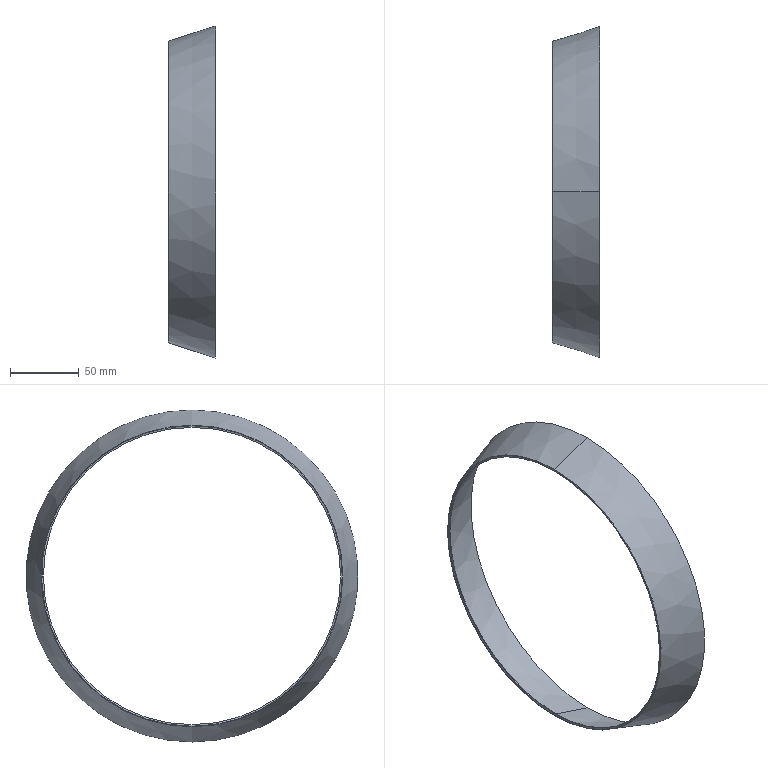Part | SolidWorks | features BaseBody 1 | 1 solid | 16 faces | box 34.434 x 242.32 x 242.32 mm | volume 26377 mm3 | cone 12 | torus 4
STEP:
#1=CARTESIAN_POINT('',(0.03978,0.,110.013));
#2=VERTEX_POINT('',#1);
#3=CARTESIAN_POINT('',(33.989,0.,121.16));
#4=VERTEX_POINT('',#3);
#5=CARTESIAN_POINT('',(0.03978,0.,110.013));
#6=DIRECTION('',(0.9501,0.,0.312));
#7=VECTOR('',#6,1000.);
#8=LINE('',#5,#7);
#9=EDGE_CURVE('',#2,#4,#8,.T.);
#10=ORIENTED_EDGE('',*,*,#9,.F.);
#11=CARTESIAN_POINT('',(0.03978,-104.628,-33.996));
#12=VERTEX_POINT('',#11);
#13=CARTESIAN_POINT('',(0.03978,0.,0.));
#14=DIRECTION('',(1.,0.,0.));
#15=DIRECTION('',(0.,0.,-1.));
#16=AXIS2_PLACEMENT_3D('',#13,#14,#15);
#17=CIRCLE('',#16,110.013);
#18=EDGE_CURVE('',#2,#12,#17,.T.);
#19=ORIENTED_EDGE('',*,*,#18,.T.);
#20=CARTESIAN_POINT('',(0.03978,0.,-110.013));
#21=VERTEX_POINT('',#20);
#22=CARTESIAN_POINT('',(0.03978,0.,0.));
#23=DIRECTION('',(1.,0.,0.));
#24=DIRECTION('',(0.,0.,-1.));
#25=AXIS2_PLACEMENT_3D('',#22,#23,#24);
#26=CIRCLE('',#25,110.013);
#27=EDGE_CURVE('',#12,#21,#26,.T.);
#28=ORIENTED_EDGE('',*,*,#27,.T.);
#29=CARTESIAN_POINT('',(33.989,0.,-121.16));
#30=VERTEX_POINT('',#29);
#31=CARTESIAN_POINT('',(0.03978,0.,-110.013));
#32=DIRECTION('',(0.9501,0.,-0.312));
#33=VECTOR('',#32,1000.);
#34=LINE('',#31,#33);
#35=EDGE_CURVE('',#21,#30,#34,.T.);
#36=ORIENTED_EDGE('',*,*,#35,.T.);
#37=CARTESIAN_POINT('',(33.989,0.,0.));
#38=DIRECTION('',(1.,0.,0.));
#39=DIRECTION('',(0.,0.,-1.));
#40=AXIS2_PLACEMENT_3D('',#37,#38,#39);
#41=CIRCLE('',#40,121.16);
#42=EDGE_CURVE('',#4,#30,#41,.T.);
#43=ORIENTED_EDGE('',*,*,#42,.F.);
#44=EDGE_LOOP('',(#10,#19,#28,#36,#43));
#45=FACE_OUTER_BOUND('',#44,.T.);
#46=CARTESIAN_POINT('',(33.989,0.,0.));
#47=DIRECTION('',(1.,0.,0.));
#48=DIRECTION('',(0.,1.,0.));
#49=AXIS2_PLACEMENT_3D('',#46,#47,#48);
#50=CONICAL_SURFACE('',#49,121.16,0.3173);
#51=ADVANCED_FACE('',(#45),#50,.T.);
#52=CARTESIAN_POINT('',(34.268,0.,-120.199));
#53=VERTEX_POINT('',#52);
#54=CARTESIAN_POINT('',(34.268,0.,-120.199));
#55=DIRECTION('',(-0.2785,0.,-0.9604));
#56=VECTOR('',#55,1000.);
#57=LINE('',#54,#56);
#58=EDGE_CURVE('',#53,#30,#57,.T.);
#59=ORIENTED_EDGE('',*,*,#58,.F.);
#60=CARTESIAN_POINT('',(34.268,0.,120.199));
#61=VERTEX_POINT('',#60);
#62=CARTESIAN_POINT('',(34.268,0.,0.));
#63=DIRECTION('',(1.,0.,0.));
#64=DIRECTION('',(0.,0.,-1.));
#65=AXIS2_PLACEMENT_3D('',#62,#63,#64);
#66=CIRCLE('',#65,120.199);
#67=EDGE_CURVE('',#61,#53,#66,.T.);
#68=ORIENTED_EDGE('',*,*,#67,.F.);
#69=CARTESIAN_POINT('',(34.268,0.,120.199));
#70=DIRECTION('',(-0.2785,0.,0.9604));
#71=VECTOR('',#70,1000.);
#72=LINE('',#69,#71);
#73=EDGE_CURVE('',#61,#4,#72,.T.);
#74=ORIENTED_EDGE('',*,*,#73,.T.);
#75=ORIENTED_EDGE('',*,*,#42,.T.);
#76=EDGE_LOOP('',(#59,#68,#74,#75));
#77=FACE_OUTER_BOUND('',#76,.T.);
#78=CARTESIAN_POINT('',(34.268,0.,0.));
#79=DIRECTION('',(-1.,0.,0.));
#80=DIRECTION('',(0.,1.,0.));
#81=AXIS2_PLACEMENT_3D('',#78,#79,#80);
#82=CONICAL_SURFACE('',#81,120.199,1.289);
#83=ADVANCED_FACE('',(#77),#82,.T.);
#84=ORIENTED_EDGE('',*,*,#58,.T.);
#85=CARTESIAN_POINT('',(33.989,0.,0.));
#86=DIRECTION('',(1.,0.,0.));
#87=DIRECTION('',(0.,0.,-1.));
#88=AXIS2_PLACEMENT_3D('',#85,#86,#87);
#89=CIRCLE('',#88,121.16);
#90=EDGE_CURVE('',#30,#4,#89,.T.);
#91=ORIENTED_EDGE('',*,*,#90,.T.);
#92=ORIENTED_EDGE('',*,*,#73,.F.);
#93=CARTESIAN_POINT('',(34.268,0.,0.));
#94=DIRECTION('',(1.,0.,0.));
#95=DIRECTION('',(0.,0.,-1.));
#96=AXIS2_PLACEMENT_3D('',#93,#94,#95);
#97=CIRCLE('',#96,120.199);
#98=EDGE_CURVE('',#53,#61,#97,.T.);
#99=ORIENTED_EDGE('',*,*,#98,.F.);
#100=EDGE_LOOP('',(#84,#91,#92,#99));
#101=FACE_OUTER_BOUND('',#100,.T.);
#102=CARTESIAN_POINT('',(34.268,0.,0.));
#103=DIRECTION('',(-1.,0.,0.));
#104=DIRECTION('',(0.,-1.,0.));
#105=AXIS2_PLACEMENT_3D('',#102,#103,#104);
#106=CONICAL_SURFACE('',#105,120.199,1.289);
#107=ADVANCED_FACE('',(#101),#106,.T.);
#108=CARTESIAN_POINT('',(1.177,0.,109.334));
#109=VERTEX_POINT('',#108);
#110=CARTESIAN_POINT('',(1.177,0.,109.334));
#111=DIRECTION('',(0.9501,0.,0.312));
#112=VECTOR('',#111,1000.);
#113=LINE('',#110,#112);
#114=EDGE_CURVE('',#109,#61,#113,.T.);
#115=ORIENTED_EDGE('',*,*,#114,.F.);
#116=CARTESIAN_POINT('',(1.177,103.983,33.786));
#117=VERTEX_POINT('',#116);
#118=CARTESIAN_POINT('',(1.177,0.,0.));
#119=DIRECTION('',(1.,0.,0.));
#120=DIRECTION('',(0.,0.,-1.));
#121=AXIS2_PLACEMENT_3D('',#118,#119,#120);
#122=CIRCLE('',#121,109.334);
#123=EDGE_CURVE('',#117,#109,#122,.T.);
#124=ORIENTED_EDGE('',*,*,#123,.F.);
#125=CARTESIAN_POINT('',(1.177,0.,-109.334));
#126=VERTEX_POINT('',#125);
#127=CARTESIAN_POINT('',(1.177,0.,0.));
#128=DIRECTION('',(1.,0.,0.));
#129=DIRECTION('',(0.,0.,-1.));
#130=AXIS2_PLACEMENT_3D('',#127,#128,#129);
#131=CIRCLE('',#130,109.334);
#132=EDGE_CURVE('',#126,#117,#131,.T.);
#133=ORIENTED_EDGE('',*,*,#132,.F.);
#134=CARTESIAN_POINT('',(1.177,0.,-109.334));
#135=DIRECTION('',(0.9501,0.,-0.312));
#136=VECTOR('',#135,1000.);
#137=LINE('',#134,#136);
#138=EDGE_CURVE('',#126,#53,#137,.T.);
#139=ORIENTED_EDGE('',*,*,#138,.T.);
#140=ORIENTED_EDGE('',*,*,#98,.T.);
#141=EDGE_LOOP('',(#115,#124,#133,#139,#140));
#142=FACE_OUTER_BOUND('',#141,.T.);
#143=CARTESIAN_POINT('',(1.177,0.,0.));
#144=DIRECTION('',(1.,0.,0.));
#145=DIRECTION('',(0.,-1.,0.));
#146=AXIS2_PLACEMENT_3D('',#143,#144,#145);
#147=CONICAL_SURFACE('',#146,109.334,0.3173);
#148=ADVANCED_FACE('',(#142),#147,.F.);
#149=ORIENTED_EDGE('',*,*,#114,.T.);
#150=ORIENTED_EDGE('',*,*,#67,.T.);
#151=ORIENTED_EDGE('',*,*,#138,.F.);
#152=CARTESIAN_POINT('',(1.177,-103.983,-33.786));
#153=VERTEX_POINT('',#152);
#154=CARTESIAN_POINT('',(1.177,0.,0.));
#155=DIRECTION('',(1.,0.,0.));
#156=DIRECTION('',(0.,0.,-1.));
#157=AXIS2_PLACEMENT_3D('',#154,#155,#156);
#158=CIRCLE('',#157,109.334);
#159=EDGE_CURVE('',#153,#126,#158,.T.);
#160=ORIENTED_EDGE('',*,*,#159,.F.);
#161=CARTESIAN_POINT('',(1.177,0.,0.));
#162=DIRECTION('',(1.,0.,0.));
#163=DIRECTION('',(0.,0.,-1.));
#164=AXIS2_PLACEMENT_3D('',#161,#162,#163);
#165=CIRCLE('',#164,109.334);
#166=EDGE_CURVE('',#109,#153,#165,.T.);
#167=ORIENTED_EDGE('',*,*,#166,.F.);
#168=EDGE_LOOP('',(#149,#150,#151,#160,#167));
#169=FACE_OUTER_BOUND('',#168,.T.);
#170=CARTESIAN_POINT('',(1.177,0.,0.));
#171=DIRECTION('',(1.,0.,0.));
#172=DIRECTION('',(0.,1.,0.));
#173=AXIS2_PLACEMENT_3D('',#170,#171,#172);
#174=CONICAL_SURFACE('',#173,109.334,0.3173);
#175=ADVANCED_FACE('',(#169),#174,.F.);
#176=CARTESIAN_POINT('',(1.048,-103.749,-33.71));
#177=VERTEX_POINT('',#176);
#178=CARTESIAN_POINT('',(1.24,-103.802,-33.727));
#179=DIRECTION('',(0.,0.309,-0.9511));
#180=DIRECTION('',(-0.312,-0.9036,-0.2936));
#181=AXIS2_PLACEMENT_3D('',#178,#179,#180);
#182=CIRCLE('',#181,0.2);
#183=EDGE_CURVE('',#153,#177,#182,.T.);
#184=ORIENTED_EDGE('',*,*,#183,.T.);
#185=CARTESIAN_POINT('',(1.048,0.,109.088));
#186=VERTEX_POINT('',#185);
#187=CARTESIAN_POINT('',(1.048,0.,109.088));
#188=CARTESIAN_POINT('',(1.048,-8.568,109.088));
#189=CARTESIAN_POINT('',(1.048,-17.135,108.074));
#190=CARTESIAN_POINT('',(1.048,-33.797,104.074));
#191=CARTESIAN_POINT('',(1.048,-41.891,101.088));
#192=CARTESIAN_POINT('',(1.048,-57.159,93.308));
#193=CARTESIAN_POINT('',(1.048,-64.332,88.515));
#194=CARTESIAN_POINT('',(1.048,-77.362,77.387));
#195=CARTESIAN_POINT('',(1.048,-83.218,71.052));
#196=CARTESIAN_POINT('',(1.048,-93.29,57.189));
#197=CARTESIAN_POINT('',(1.048,-97.505,49.662));
#198=CARTESIAN_POINT('',(1.048,-104.063,33.831));
#199=CARTESIAN_POINT('',(1.048,-106.405,25.527));
#200=CARTESIAN_POINT('',(1.048,-109.085,8.603));
#201=CARTESIAN_POINT('',(1.048,-109.424,-0.01761));
#202=CARTESIAN_POINT('',(1.048,-108.079,-17.1));
#203=CARTESIAN_POINT('',(1.048,-106.396,-25.562));
#204=CARTESIAN_POINT('',(1.048,-103.749,-33.71));
#205=B_SPLINE_CURVE_WITH_KNOTS('',3,(#187,#188,#189,#190,#191,#192,#193,#194,#195,#196,#197,#198,#199,#200,#201,#202,#203,#204),.UNSPECIFIED.,.F.,.F.,(4,2,2,2,2,2,2,2,4),(0.,0.2356,0.4712,0.7069,0.9425,1.178,1.414,1.649,1.885),.UNSPECIFIED.);
#206=EDGE_CURVE('',#186,#177,#205,.T.);
#207=ORIENTED_EDGE('',*,*,#206,.F.);
#208=CARTESIAN_POINT('',(1.048,103.749,33.71));
#209=VERTEX_POINT('',#208);
#210=CARTESIAN_POINT('',(1.048,103.749,33.71));
#211=CARTESIAN_POINT('',(1.048,101.984,39.142));
#212=CARTESIAN_POINT('',(1.048,99.791,44.436));
#213=CARTESIAN_POINT('',(1.048,94.605,54.614));
#214=CARTESIAN_POINT('',(1.048,91.611,59.499));
#215=CARTESIAN_POINT('',(1.048,84.897,68.741));
#216=CARTESIAN_POINT('',(1.048,81.176,73.098));
#217=CARTESIAN_POINT('',(1.048,73.098,81.176));
#218=CARTESIAN_POINT('',(1.048,68.741,84.897));
#219=CARTESIAN_POINT('',(1.048,59.499,91.611));
#220=CARTESIAN_POINT('',(1.048,54.614,94.605));
#221=CARTESIAN_POINT('',(1.048,44.436,99.791));
#222=CARTESIAN_POINT('',(1.048,39.142,101.984));
#223=CARTESIAN_POINT('',(1.048,28.278,105.514));
#224=CARTESIAN_POINT('',(1.048,22.707,106.851));
#225=CARTESIAN_POINT('',(1.048,11.424,108.638));
#226=CARTESIAN_POINT('',(1.048,5.712,109.088));
#227=CARTESIAN_POINT('',(1.048,0.,109.088));
#228=B_SPLINE_CURVE_WITH_KNOTS('',3,(#210,#211,#212,#213,#214,#215,#216,#217,#218,#219,#220,#221,#222,#223,#224,#225,#226,#227),.UNSPECIFIED.,.F.,.F.,(4,2,2,2,2,2,2,2,4),(0.,0.1571,0.3142,0.4712,0.6283,0.7854,0.9425,1.1,1.257),.UNSPECIFIED.);
#229=EDGE_CURVE('',#209,#186,#228,.T.);
#230=ORIENTED_EDGE('',*,*,#229,.F.);
#231=CARTESIAN_POINT('',(1.24,103.802,33.727));
#232=DIRECTION('',(0.,-0.309,0.9511));
#233=DIRECTION('',(-0.312,0.9036,0.2936));
#234=AXIS2_PLACEMENT_3D('',#231,#232,#233);
#235=CIRCLE('',#234,0.2);
#236=EDGE_CURVE('',#117,#209,#235,.T.);
#237=ORIENTED_EDGE('',*,*,#236,.F.);
#238=ORIENTED_EDGE('',*,*,#123,.T.);
#239=ORIENTED_EDGE('',*,*,#166,.T.);
#240=EDGE_LOOP('',(#184,#207,#230,#237,#238,#239));
#241=FACE_OUTER_BOUND('',#240,.T.);
#242=CARTESIAN_POINT('',(1.24,0.,0.));
#243=DIRECTION('',(1.,0.,0.));
#244=DIRECTION('',(0.,0.309,-0.9511));
#245=AXIS2_PLACEMENT_3D('',#242,#243,#244);
#246=TOROIDAL_SURFACE('',#245,109.144,0.2);
#247=ADVANCED_FACE('',(#241),#246,.F.);
#248=ORIENTED_EDGE('',*,*,#183,.F.);
#249=ORIENTED_EDGE('',*,*,#159,.T.);
#250=ORIENTED_EDGE('',*,*,#132,.T.);
#251=ORIENTED_EDGE('',*,*,#236,.T.);
#252=CARTESIAN_POINT('',(1.048,0.,-109.088));
#253=VERTEX_POINT('',#252);
#254=CARTESIAN_POINT('',(1.048,0.,0.));
#255=DIRECTION('',(1.,0.,0.));
#256=DIRECTION('',(0.,0.,-1.));
#257=AXIS2_PLACEMENT_3D('',#254,#255,#256);
#258=CIRCLE('',#257,109.088);
#259=EDGE_CURVE('',#253,#209,#258,.T.);
#260=ORIENTED_EDGE('',*,*,#259,.F.);
#261=CARTESIAN_POINT('',(1.048,-103.749,-33.71));
#262=CARTESIAN_POINT('',(1.048,-101.984,-39.142));
#263=CARTESIAN_POINT('',(1.048,-99.791,-44.436));
#264=CARTESIAN_POINT('',(1.048,-94.605,-54.614));
#265=CARTESIAN_POINT('',(1.048,-91.611,-59.499));
#266=CARTESIAN_POINT('',(1.048,-84.897,-68.741));
#267=CARTESIAN_POINT('',(1.048,-81.176,-73.098));
#268=CARTESIAN_POINT('',(1.048,-73.098,-81.176));
#269=CARTESIAN_POINT('',(1.048,-68.741,-84.897));
#270=CARTESIAN_POINT('',(1.048,-59.499,-91.611));
#271=CARTESIAN_POINT('',(1.048,-54.614,-94.605));
#272=CARTESIAN_POINT('',(1.048,-44.436,-99.791));
#273=CARTESIAN_POINT('',(1.048,-39.142,-101.984));
#274=CARTESIAN_POINT('',(1.048,-28.278,-105.514));
#275=CARTESIAN_POINT('',(1.048,-22.707,-106.851));
#276=CARTESIAN_POINT('',(1.048,-11.424,-108.638));
#277=CARTESIAN_POINT('',(1.048,-5.712,-109.088));
#278=CARTESIAN_POINT('',(1.048,0.,-109.088));
#279=B_SPLINE_CURVE_WITH_KNOTS('',3,(#261,#262,#263,#264,#265,#266,#267,#268,#269,#270,#271,#272,#273,#274,#275,#276,#277,#278),.UNSPECIFIED.,.F.,.F.,(4,2,2,2,2,2,2,2,4),(0.,0.1571,0.3142,0.4712,0.6283,0.7854,0.9425,1.1,1.257),.UNSPECIFIED.);
#280=EDGE_CURVE('',#177,#253,#279,.T.);
#281=ORIENTED_EDGE('',*,*,#280,.F.);
#282=EDGE_LOOP('',(#248,#249,#250,#251,#260,#281));
#283=FACE_OUTER_BOUND('',#282,.T.);
#284=CARTESIAN_POINT('',(1.24,0.,0.));
#285=DIRECTION('',(1.,0.,0.));
#286=DIRECTION('',(0.,-0.309,0.9511));
#287=AXIS2_PLACEMENT_3D('',#284,#285,#286);
#288=TOROIDAL_SURFACE('',#287,109.144,0.2);
#289=ADVANCED_FACE('',(#283),#288,.F.);
#290=CARTESIAN_POINT('',(1.133,0.,-108.793));
#291=VERTEX_POINT('',#290);
#292=CARTESIAN_POINT('',(1.133,0.,-108.793));
#293=DIRECTION('',(-0.2785,0.,-0.9604));
#294=VECTOR('',#293,1000.);
#295=LINE('',#292,#294);
#296=EDGE_CURVE('',#291,#253,#295,.T.);
#297=ORIENTED_EDGE('',*,*,#296,.F.);
#298=CARTESIAN_POINT('',(1.133,0.,108.793));
#299=VERTEX_POINT('',#298);
#300=CARTESIAN_POINT('',(1.133,0.,0.));
#301=DIRECTION('',(1.,0.,0.));
#302=DIRECTION('',(0.,0.,-1.));
#303=AXIS2_PLACEMENT_3D('',#300,#301,#302);
#304=CIRCLE('',#303,108.793);
#305=EDGE_CURVE('',#299,#291,#304,.T.);
#306=ORIENTED_EDGE('',*,*,#305,.F.);
#307=CARTESIAN_POINT('',(1.133,0.,108.793));
#308=DIRECTION('',(-0.2785,0.,0.9604));
#309=VECTOR('',#308,1000.);
#310=LINE('',#307,#309);
#311=EDGE_CURVE('',#299,#186,#310,.T.);
#312=ORIENTED_EDGE('',*,*,#311,.T.);
#313=ORIENTED_EDGE('',*,*,#206,.T.);
#314=ORIENTED_EDGE('',*,*,#280,.T.);
#315=EDGE_LOOP('',(#297,#306,#312,#313,#314));
#316=FACE_OUTER_BOUND('',#315,.T.);
#317=CARTESIAN_POINT('',(1.133,0.,0.));
#318=DIRECTION('',(-1.,0.,0.));
#319=DIRECTION('',(0.,1.,0.));
#320=AXIS2_PLACEMENT_3D('',#317,#318,#319);
#321=CONICAL_SURFACE('',#320,108.793,1.289);
#322=ADVANCED_FACE('',(#316),#321,.T.);
#323=ORIENTED_EDGE('',*,*,#296,.T.);
#324=ORIENTED_EDGE('',*,*,#259,.T.);
#325=ORIENTED_EDGE('',*,*,#229,.T.);
#326=ORIENTED_EDGE('',*,*,#311,.F.);
#327=CARTESIAN_POINT('',(1.133,0.,0.));
#328=DIRECTION('',(1.,0.,0.));
#329=DIRECTION('',(0.,0.,-1.));
#330=AXIS2_PLACEMENT_3D('',#327,#328,#329);
#331=CIRCLE('',#330,108.793);
#332=EDGE_CURVE('',#291,#299,#331,.T.);
#333=ORIENTED_EDGE('',*,*,#332,.F.);
#334=EDGE_LOOP('',(#323,#324,#325,#326,#333));
#335=FACE_OUTER_BOUND('',#334,.T.);
#336=CARTESIAN_POINT('',(1.133,0.,0.));
#337=DIRECTION('',(-1.,0.,0.));
#338=DIRECTION('',(0.,-1.,0.));
#339=AXIS2_PLACEMENT_3D('',#336,#337,#338);
#340=CONICAL_SURFACE('',#339,108.793,1.289);
#341=ADVANCED_FACE('',(#335),#340,.T.);
#342=CARTESIAN_POINT('',(0.1826,0.,108.481));
#343=VERTEX_POINT('',#342);
#344=CARTESIAN_POINT('',(0.1826,0.,108.481));
#345=DIRECTION('',(0.9501,0.,0.312));
#346=VECTOR('',#345,1000.);
#347=LINE('',#344,#346);
#348=EDGE_CURVE('',#343,#299,#347,.T.);
#349=ORIENTED_EDGE('',*,*,#348,.F.);
#350=CARTESIAN_POINT('',(0.1826,0.,-108.481));
#351=VERTEX_POINT('',#350);
#352=CARTESIAN_POINT('',(0.1826,0.,0.));
#353=DIRECTION('',(1.,0.,0.));
#354=DIRECTION('',(0.,0.,-1.));
#355=AXIS2_PLACEMENT_3D('',#352,#353,#354);
#356=CIRCLE('',#355,108.481);
#357=EDGE_CURVE('',#351,#343,#356,.T.);
#358=ORIENTED_EDGE('',*,*,#357,.F.);
#359=CARTESIAN_POINT('',(0.1826,0.,-108.481));
#360=DIRECTION('',(0.9501,0.,-0.312));
#361=VECTOR('',#360,1000.);
#362=LINE('',#359,#361);
#363=EDGE_CURVE('',#351,#291,#362,.T.);
#364=ORIENTED_EDGE('',*,*,#363,.T.);
#365=ORIENTED_EDGE('',*,*,#332,.T.);
#366=EDGE_LOOP('',(#349,#358,#364,#365));
#367=FACE_OUTER_BOUND('',#366,.T.);
#368=CARTESIAN_POINT('',(0.1826,0.,0.));
#369=DIRECTION('',(1.,0.,0.));
#370=DIRECTION('',(0.,-1.,0.));
#371=AXIS2_PLACEMENT_3D('',#368,#369,#370);
#372=CONICAL_SURFACE('',#371,108.481,0.3173);
#373=ADVANCED_FACE('',(#367),#372,.F.);
#374=ORIENTED_EDGE('',*,*,#348,.T.);
#375=ORIENTED_EDGE('',*,*,#305,.T.);
#376=ORIENTED_EDGE('',*,*,#363,.F.);
#377=CARTESIAN_POINT('',(0.1826,0.,0.));
#378=DIRECTION('',(1.,0.,0.));
#379=DIRECTION('',(0.,0.,-1.));
#380=AXIS2_PLACEMENT_3D('',#377,#378,#379);
#381=CIRCLE('',#380,108.481);
#382=EDGE_CURVE('',#343,#351,#381,.T.);
#383=ORIENTED_EDGE('',*,*,#382,.F.);
#384=EDGE_LOOP('',(#374,#375,#376,#383));
#385=FACE_OUTER_BOUND('',#384,.T.);
#386=CARTESIAN_POINT('',(0.1826,0.,0.));
#387=DIRECTION('',(1.,0.,0.));
#388=DIRECTION('',(0.,1.,0.));
#389=AXIS2_PLACEMENT_3D('',#386,#387,#388);
#390=CONICAL_SURFACE('',#389,108.481,0.3173);
#391=ADVANCED_FACE('',(#385),#390,.F.);
#392=CARTESIAN_POINT('',(-0.1548,0.,-109.644));
#393=VERTEX_POINT('',#392);
#394=CARTESIAN_POINT('',(0.1826,0.,-108.481));
#395=DIRECTION('',(-0.2785,0.,-0.9604));
#396=VECTOR('',#395,1000.);
#397=LINE('',#394,#396);
#398=EDGE_CURVE('',#351,#393,#397,.T.);
#399=ORIENTED_EDGE('',*,*,#398,.T.);
#400=CARTESIAN_POINT('',(-0.1548,-104.278,-33.882));
#401=VERTEX_POINT('',#400);
#402=CARTESIAN_POINT('',(-0.1548,-104.278,-33.882));
#403=CARTESIAN_POINT('',(-0.1548,-102.504,-39.342));
#404=CARTESIAN_POINT('',(-0.1548,-100.3,-44.662));
#405=CARTESIAN_POINT('',(-0.1548,-95.087,-54.893));
#406=CARTESIAN_POINT('',(-0.1548,-92.078,-59.803));
#407=CARTESIAN_POINT('',(-0.1548,-85.329,-69.092));
#408=CARTESIAN_POINT('',(-0.1548,-81.59,-73.471));
#409=CARTESIAN_POINT('',(-0.1548,-73.471,-81.59));
#410=CARTESIAN_POINT('',(-0.1548,-69.092,-85.329));
#411=CARTESIAN_POINT('',(-0.1548,-59.803,-92.078));
#412=CARTESIAN_POINT('',(-0.1548,-54.893,-95.087));
#413=CARTESIAN_POINT('',(-0.1548,-44.662,-100.3));
#414=CARTESIAN_POINT('',(-0.1548,-39.342,-102.504));
#415=CARTESIAN_POINT('',(-0.1548,-28.422,-106.052));
#416=CARTESIAN_POINT('',(-0.1548,-22.822,-107.396));
#417=CARTESIAN_POINT('',(-0.1548,-11.482,-109.192));
#418=CARTESIAN_POINT('',(-0.1548,-5.741,-109.644));
#419=CARTESIAN_POINT('',(-0.1548,0.,-109.644));
#420=B_SPLINE_CURVE_WITH_KNOTS('',3,(#402,#403,#404,#405,#406,#407,#408,#409,#410,#411,#412,#413,#414,#415,#416,#417,#418,#419),.UNSPECIFIED.,.F.,.F.,(4,2,2,2,2,2,2,2,4),(0.,0.1571,0.3142,0.4712,0.6283,0.7854,0.9425,1.1,1.257),.UNSPECIFIED.);
#421=EDGE_CURVE('',#401,#393,#420,.T.);
#422=ORIENTED_EDGE('',*,*,#421,.F.);
#423=CARTESIAN_POINT('',(-0.1548,0.,109.644));
#424=VERTEX_POINT('',#423);
#425=CARTESIAN_POINT('',(-0.1548,0.,0.));
#426=DIRECTION('',(1.,0.,0.));
#427=DIRECTION('',(0.,0.,-1.));
#428=AXIS2_PLACEMENT_3D('',#425,#426,#427);
#429=CIRCLE('',#428,109.644);
#430=EDGE_CURVE('',#424,#401,#429,.T.);
#431=ORIENTED_EDGE('',*,*,#430,.F.);
#432=CARTESIAN_POINT('',(0.1826,0.,108.481));
#433=DIRECTION('',(-0.2785,0.,0.9604));
#434=VECTOR('',#433,1000.);
#435=LINE('',#432,#434);
#436=EDGE_CURVE('',#343,#424,#435,.T.);
#437=ORIENTED_EDGE('',*,*,#436,.F.);
#438=ORIENTED_EDGE('',*,*,#382,.T.);
#439=EDGE_LOOP('',(#399,#422,#431,#437,#438));
#440=FACE_OUTER_BOUND('',#439,.T.);
#441=CARTESIAN_POINT('',(-0.1548,0.,0.));
#442=DIRECTION('',(-1.,0.,0.));
#443=DIRECTION('',(0.,1.,0.));
#444=AXIS2_PLACEMENT_3D('',#441,#442,#443);
#445=CONICAL_SURFACE('',#444,109.644,1.289);
#446=ADVANCED_FACE('',(#440),#445,.F.);
#447=ORIENTED_EDGE('',*,*,#398,.F.);
#448=ORIENTED_EDGE('',*,*,#357,.T.);
#449=ORIENTED_EDGE('',*,*,#436,.T.);
#450=CARTESIAN_POINT('',(-0.1548,104.278,33.882));
#451=VERTEX_POINT('',#450);
#452=CARTESIAN_POINT('',(-0.1548,104.278,33.882));
#453=CARTESIAN_POINT('',(-0.1548,102.504,39.342));
#454=CARTESIAN_POINT('',(-0.1548,100.3,44.662));
#455=CARTESIAN_POINT('',(-0.1548,95.087,54.893));
#456=CARTESIAN_POINT('',(-0.1548,92.078,59.803));
#457=CARTESIAN_POINT('',(-0.1548,85.329,69.092));
#458=CARTESIAN_POINT('',(-0.1548,81.59,73.471));
#459=CARTESIAN_POINT('',(-0.1548,73.471,81.59));
#460=CARTESIAN_POINT('',(-0.1548,69.092,85.329));
#461=CARTESIAN_POINT('',(-0.1548,59.803,92.078));
#462=CARTESIAN_POINT('',(-0.1548,54.893,95.087));
#463=CARTESIAN_POINT('',(-0.1548,44.662,100.3));
#464=CARTESIAN_POINT('',(-0.1548,39.342,102.504));
#465=CARTESIAN_POINT('',(-0.1548,28.422,106.052));
#466=CARTESIAN_POINT('',(-0.1548,22.822,107.396));
#467=CARTESIAN_POINT('',(-0.1548,11.482,109.192));
#468=CARTESIAN_POINT('',(-0.1548,5.741,109.644));
#469=CARTESIAN_POINT('',(-0.1548,0.,109.644));
#470=B_SPLINE_CURVE_WITH_KNOTS('',3,(#452,#453,#454,#455,#456,#457,#458,#459,#460,#461,#462,#463,#464,#465,#466,#467,#468,#469),.UNSPECIFIED.,.F.,.F.,(4,2,2,2,2,2,2,2,4),(0.,0.1571,0.3142,0.4712,0.6283,0.7854,0.9425,1.1,1.257),.UNSPECIFIED.);
#471=EDGE_CURVE('',#451,#424,#470,.T.);
#472=ORIENTED_EDGE('',*,*,#471,.F.);
#473=CARTESIAN_POINT('',(-0.1548,0.,-109.644));
#474=CARTESIAN_POINT('',(-0.1548,8.611,-109.644));
#475=CARTESIAN_POINT('',(-0.1548,17.222,-108.625));
#476=CARTESIAN_POINT('',(-0.1548,33.969,-104.604));
#477=CARTESIAN_POINT('',(-0.1548,42.105,-101.603));
#478=CARTESIAN_POINT('',(-0.1548,57.45,-93.784));
#479=CARTESIAN_POINT('',(-0.1548,64.66,-88.967));
#480=CARTESIAN_POINT('',(-0.1548,77.756,-77.781));
#481=CARTESIAN_POINT('',(-0.1548,83.642,-71.414));
#482=CARTESIAN_POINT('',(-0.1548,93.766,-57.48));
#483=CARTESIAN_POINT('',(-0.1548,98.002,-49.915));
#484=CARTESIAN_POINT('',(-0.1548,104.593,-34.003));
#485=CARTESIAN_POINT('',(-0.1548,106.947,-25.658));
#486=CARTESIAN_POINT('',(-0.1548,109.641,-8.647));
#487=CARTESIAN_POINT('',(-0.1548,109.982,0.0177));
#488=CARTESIAN_POINT('',(-0.1548,108.63,17.187));
#489=CARTESIAN_POINT('',(-0.1548,106.939,25.692));
#490=CARTESIAN_POINT('',(-0.1548,104.278,33.882));
#491=B_SPLINE_CURVE_WITH_KNOTS('',3,(#473,#474,#475,#476,#477,#478,#479,#480,#481,#482,#483,#484,#485,#486,#487,#488,#489,#490),.UNSPECIFIED.,.F.,.F.,(4,2,2,2,2,2,2,2,4),(0.,0.2356,0.4712,0.7069,0.9425,1.178,1.414,1.649,1.885),.UNSPECIFIED.);
#492=EDGE_CURVE('',#393,#451,#491,.T.);
#493=ORIENTED_EDGE('',*,*,#492,.F.);
#494=EDGE_LOOP('',(#447,#448,#449,#472,#493));
#495=FACE_OUTER_BOUND('',#494,.T.);
#496=CARTESIAN_POINT('',(-0.1548,0.,0.));
#497=DIRECTION('',(-1.,0.,0.));
#498=DIRECTION('',(0.,-1.,0.));
#499=AXIS2_PLACEMENT_3D('',#496,#497,#498);
#500=CONICAL_SURFACE('',#499,109.644,1.289);
#501=ADVANCED_FACE('',(#495),#500,.F.);
#502=CARTESIAN_POINT('',(0.1334,-104.357,-33.908));
#503=DIRECTION('',(0.,0.309,-0.9511));
#504=DIRECTION('',(-0.312,-0.9036,-0.2936));
#505=AXIS2_PLACEMENT_3D('',#502,#503,#504);
#506=CIRCLE('',#505,0.3);
#507=EDGE_CURVE('',#12,#401,#506,.T.);
#508=ORIENTED_EDGE('',*,*,#507,.T.);
#509=ORIENTED_EDGE('',*,*,#421,.T.);
#510=ORIENTED_EDGE('',*,*,#492,.T.);
#511=CARTESIAN_POINT('',(0.03978,104.628,33.996));
#512=VERTEX_POINT('',#511);
#513=CARTESIAN_POINT('',(0.1334,104.357,33.908));
#514=DIRECTION('',(0.,-0.309,0.9511));
#515=DIRECTION('',(-0.312,0.9036,0.2936));
#516=AXIS2_PLACEMENT_3D('',#513,#514,#515);
#517=CIRCLE('',#516,0.3);
#518=EDGE_CURVE('',#512,#451,#517,.T.);
#519=ORIENTED_EDGE('',*,*,#518,.F.);
#520=CARTESIAN_POINT('',(0.03978,0.,0.));
#521=DIRECTION('',(1.,0.,0.));
#522=DIRECTION('',(0.,0.,-1.));
#523=AXIS2_PLACEMENT_3D('',#520,#521,#522);
#524=CIRCLE('',#523,110.013);
#525=EDGE_CURVE('',#21,#512,#524,.T.);
#526=ORIENTED_EDGE('',*,*,#525,.F.);
#527=ORIENTED_EDGE('',*,*,#27,.F.);
#528=EDGE_LOOP('',(#508,#509,#510,#519,#526,#527));
#529=FACE_OUTER_BOUND('',#528,.T.);
#530=CARTESIAN_POINT('',(0.1334,0.,0.));
#531=DIRECTION('',(1.,0.,0.));
#532=DIRECTION('',(0.,-0.309,0.9511));
#533=AXIS2_PLACEMENT_3D('',#530,#531,#532);
#534=TOROIDAL_SURFACE('',#533,109.728,0.3);
#535=ADVANCED_FACE('',(#529),#534,.T.);
#536=ORIENTED_EDGE('',*,*,#9,.T.);
#537=ORIENTED_EDGE('',*,*,#90,.F.);
#538=ORIENTED_EDGE('',*,*,#35,.F.);
#539=ORIENTED_EDGE('',*,*,#525,.T.);
#540=CARTESIAN_POINT('',(0.03978,0.,0.));
#541=DIRECTION('',(1.,0.,0.));
#542=DIRECTION('',(0.,0.,-1.));
#543=AXIS2_PLACEMENT_3D('',#540,#541,#542);
#544=CIRCLE('',#543,110.013);
#545=EDGE_CURVE('',#512,#2,#544,.T.);
#546=ORIENTED_EDGE('',*,*,#545,.T.);
#547=EDGE_LOOP('',(#536,#537,#538,#539,#546));
#548=FACE_OUTER_BOUND('',#547,.T.);
#549=CARTESIAN_POINT('',(33.989,0.,0.));
#550=DIRECTION('',(1.,0.,0.));
#551=DIRECTION('',(0.,-1.,0.));
#552=AXIS2_PLACEMENT_3D('',#549,#550,#551);
#553=CONICAL_SURFACE('',#552,121.16,0.3173);
#554=ADVANCED_FACE('',(#548),#553,.T.);
#555=ORIENTED_EDGE('',*,*,#507,.F.);
#556=ORIENTED_EDGE('',*,*,#18,.F.);
#557=ORIENTED_EDGE('',*,*,#545,.F.);
#558=ORIENTED_EDGE('',*,*,#518,.T.);
#559=ORIENTED_EDGE('',*,*,#471,.T.);
#560=ORIENTED_EDGE('',*,*,#430,.T.);
#561=EDGE_LOOP('',(#555,#556,#557,#558,#559,#560));
#562=FACE_OUTER_BOUND('',#561,.T.);
#563=CARTESIAN_POINT('',(0.1334,0.,0.));
#564=DIRECTION('',(1.,0.,0.));
#565=DIRECTION('',(0.,0.309,-0.9511));
#566=AXIS2_PLACEMENT_3D('',#563,#564,#565);
#567=TOROIDAL_SURFACE('',#566,109.728,0.3);
#568=ADVANCED_FACE('',(#562),#567,.T.);
#569=CLOSED_SHELL('',(#51,#83,#107,#148,#175,#247,#289,#322,#341,#373,#391,#446,#501,#535,#554,#568));
#570=MANIFOLD_SOLID_BREP('',#569);
#571=CARTESIAN_POINT('',(0.,0.,0.));
#572=DIRECTION('',(0.,0.,1.));
#573=DIRECTION('',(1.,0.,0.));
#574=AXIS2_PLACEMENT_3D('',#571,#572,#573);
#575=(LENGTH_UNIT()NAMED_UNIT(*)SI_UNIT(.MILLI.,.METRE.));
#576=UNCERTAINTY_MEASURE_WITH_UNIT(LENGTH_MEASURE(0.00001),#575,'','');
#577=(NAMED_UNIT(*)PLANE_ANGLE_UNIT()SI_UNIT($,.RADIAN.));
#578=(NAMED_UNIT(*)SI_UNIT($,.STERADIAN.)SOLID_ANGLE_UNIT());
#579=(GEOMETRIC_REPRESENTATION_CONTEXT(3)GLOBAL_UNCERTAINTY_ASSIGNED_CONTEXT((#576))GLOBAL_UNIT_ASSIGNED_CONTEXT((#575,#577,#578))REPRESENTATION_CONTEXT('',''));
#580=ADVANCED_BREP_SHAPE_REPRESENTATION('',(#570,#574),#579);